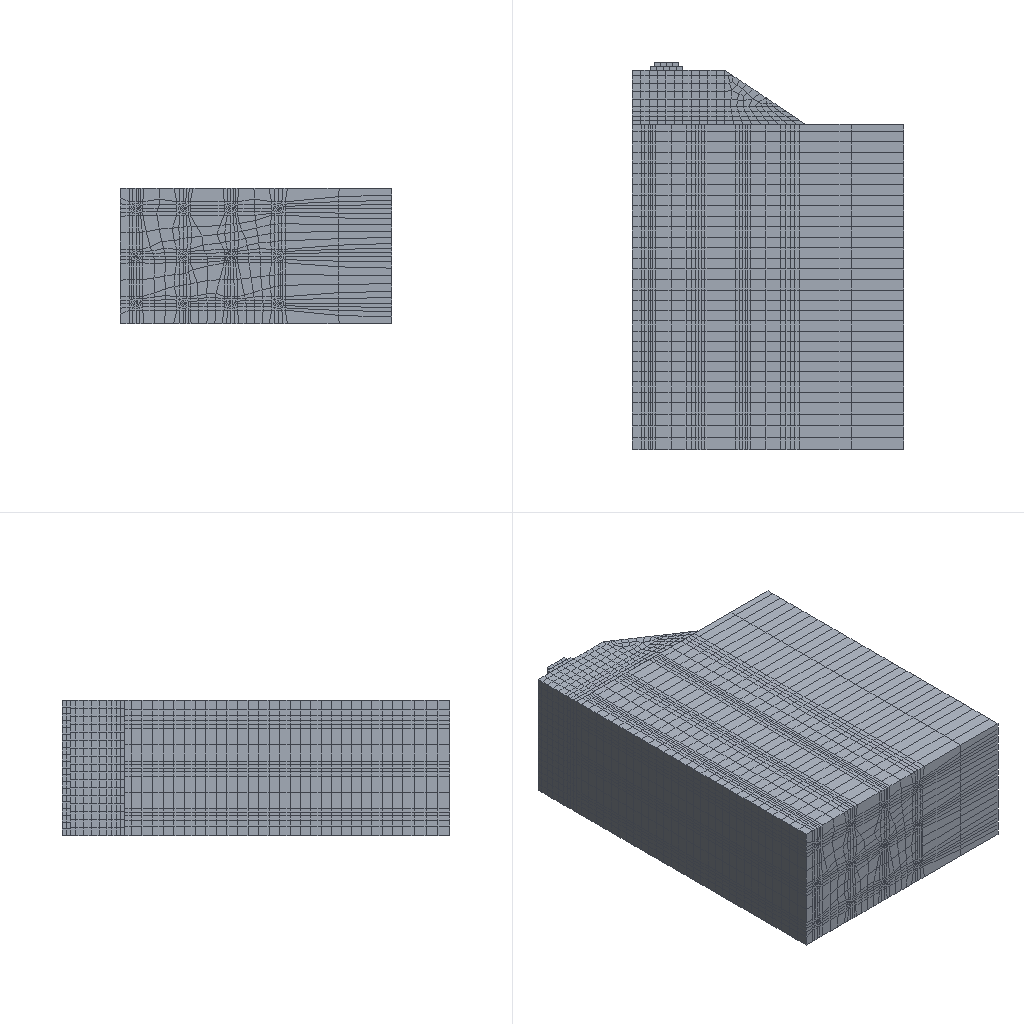Simulation study | abaqus
Set-up summary:
category,name,step,type,value,unit,region
solver,abaqus
solver,version,,,Abaqus/Standard 2020
units,not stated in the deck,,not stated
analysis,deck,,geostatic,geostatic
load_step,Step-geo,Step-geo,geostatic
load_step,Step-ludi,Step-ludi,static
load_step,Step-load,Step-load,static
load_step,requested,,,3
mesh,nodes,,,32812
mesh,elements,,,26703
element_type,C3D8R,,solid,26623
element_type,M3D4R,,membrane,80
load,load commands in deck,,count,2
bc,support commands in deck,,count,3
material,DIZUOBAN,,in results
material,FENSHA,,in results
material,GESHAN,,in results
material,GUIDAOBAN,,in results
material,JICHAUNBIAOCENG,,in results
material,JICHUANDICENG,,in results
material,LUDI,,in results
material,RUANTU1,,in results
material,RUANTU2,,in results
material,RUANTU3,,in results
material,SUISHI,,in results
material,ZHUANG,,in results
check,setup vs results,,match,"per instance, exact: element labels, types and connectivity; labels of the nodes the elements use; coordinates of those nodes at SINGLE_PRECISION in 6 of 6 instance(s)"
Abaqus input file, long lists of numbers shortened:
*Heading
** Job name: Job-1 Model name: Model-1
** Generated by: Abaqus/CAE 2020
*Preprint, echo=NO, model=NO, history=NO, contact=NO
**
** PARTS
**
*Part, name=dizuoban
*Node
      1,   3.7,   4.3,          10.
      2,   3.7,           4.,          10.
** (250 more lines like these left out)
*Element, type=C3D8R
  1,  43,  44,  46,  45,   1,   2,   4,   3
  2,  45,  46,  48,  47,   3,   4,   6,   5
** (98 more lines like these left out)
*Nset, nset=Set-1, generate
   1,  252,    1
*Elset, elset=Set-1, generate
   1,  100,    1
** Section: dizuoban
*Solid Section, elset=Set-1, material=dizuoban
,
*End Part
**
*Part, name=geshan
*Node
      1,           0.,  0.3,           0.
      2,   1.235,  0.3,           0.
** (97 more lines like these left out)
*Element, type=M3D4R
 1,  1,  2, 13, 12
 2,  2,  3, 14, 13
** (78 more lines like these left out)
*Nset, nset=Set-2, generate
  1,  99,   1
*Elset, elset=Set-2, generate
  1,  80,   1
** Section: geshan
*Membrane Section, elset=Set-2, material=geshan
0.003,
*End Part
**
*Part, name=guidaoban
*Node
      1,    3.4,    4.6,          10.
      2,    3.4,   4.3,          10.
** (208 more lines like these left out)
*Element, type=C3D8R
 1,  43,  44,  46,  45,   1,   2,   4,   3
 2,  45,  46,  48,  47,   3,   4,   6,   5
** (78 more lines like these left out)
*Nset, nset=Set-1, generate
   1,  210,    1
*Elset, elset=Set-1, generate
  1,  80,   1
** Section: guidaoban
*Solid Section, elset=Set-1, material=guidaoban
,
*End Part
**
*Part, name=ludi
*Node
      1,   6.8, -0.4,           0.
      2,   6.8, -0.4,          10.
** (3400 more lines like these left out)
*Element, type=C3D8R
  1,    1,   29,  439,   80,   81,  789, 2091,  768
  2,   29,   30,  440,  439,  789,  790, 2092, 2091
** (2752 more lines like these left out)
*Nset, nset=Set-4
    1,    2,    3,    4,   17,   18,   19,   20,   26,   27,   29,   30,   31,   32,   33,   34
   35,   36,   37,   38,   39,   40,   41,   42,   43,   44,   45,   46,   47,   48,   49,   50
** (28 more lines like these left out)
*Elset, elset=Set-4
 1497, 1498, 1499, 1500, 1501, 1502, 1503, 1504, 1505, 1506, 1507, 1508, 1509, 1510, 1511, 1512
 1513, 1514, 1515, 1516, 1517, 1518, 1519, 1520, 1521, 1522, 1523, 1524, 1525, 1526, 1527, 1528
** (11 more lines like these left out)
*Nset, nset=Set-5
    1,    2,    3,    4,    5,    6,    7,    8,   25,   26,   27,   28,   29,   30,   31,   32
   33,   34,   35,   36,   37,   38,   39,   40,   41,   42,   43,   44,   45,   46,   47,   48
** (103 more lines like these left out)
*Elset, elset=Set-5
    1,    2,    3,    4,    5,    6,    7,    8,    9,   10,   11,   12,   13,   14,   15,   16
   17,   18,   19,   20,   21,   22,   23,   24,   25,   26,   27,   28,   29,   30,   31,   32
** (73 more lines like these left out)
*Nset, nset=Set-6
    5,    6,    7,    8,    9,   10,   11,   12,   21,   24,   25,   28,   93,   94,   95,   96
   97,   98,   99,  100,  101,  102,  103,  104,  105,  106,  107,  108,  109,  110,  111,  112
** (69 more lines like these left out)
*Elset, elset=Set-6
  749,  750,  751,  752,  753,  754,  755,  756,  757,  758,  759,  760,  761,  762,  763,  764
  765,  766,  767,  768,  769,  770,  771,  772,  773,  774,  775,  776,  777,  778,  779,  780
** (41 more lines like these left out)
*Nset, nset=Set-7
    9,   10,   11,   12,   13,   14,   15,   16,   21,   22,   23,   24,  149,  150,  151,  152
  153,  154,  155,  156,  157,  158,  159,  160,  161,  162,  163,  164,  165,  166,  167,  168
** (69 more lines like these left out)
*Elset, elset=Set-7
 1123, 1124, 1125, 1126, 1127, 1128, 1129, 1130, 1131, 1132, 1133, 1134, 1135, 1136, 1137, 1138
 1139, 1140, 1141, 1142, 1143, 1144, 1145, 1146, 1147, 1148, 1149, 1150, 1151, 1152, 1153, 1154
** (41 more lines like these left out)
** Section: jichuandiceng
*Solid Section, elset=Set-5, material=jichuandiceng
,
** Section: ludi
*Solid Section, elset=Set-6, material=ludi
,
** Section: suishi
*Solid Section, elset=Set-7, material=suishi
,
** Section: jichuanbiaoceng
*Solid Section, elset=Set-4, material=jichaunbiaoceng
,
*End Part
**
*Part, name=pile
*Node
      1,   8.15,           0.,           8.
      2,   8.15,           0.,         8.25
** (3514 more lines like these left out)
*Element, type=C3D8R
 1, 1647,  375, 1646, 2989,  373,    1,  374, 1645
 2, 1648,  377, 1647, 2989,  376,    2,  373, 1645
** (2206 more lines like these left out)
*Nset, nset=Set-1, generate
    1,  3516,     1
*Elset, elset=Set-1, generate
    1,  2208,     1
** Section: zhuang
*Solid Section, elset=Set-1, material=zhuang
,
*End Part
**
*Part, name=soil-merge
*Node
      1,   12.15,         -19.,          5.5
      2,   12.15,         -19.,           8.
** (25331 more lines like these left out)
*Element, type=C3D8R
  1,  1162,  7498,  7495,     1,  7544, 18528, 18525,  1218
  2,  7498,  7499,  7496,  7495, 18528, 18529, 18526, 18525
** (21479 more lines like these left out)
*Nset, nset=Set-1
     1,     2,     3,     4,     5,     8,     9,    10,    11,    12,    15,    16,    17,    18,    19,    20
    21,    22,    23,    24,    25,    26,    27,    28,    29,    30,    31,    32,    33,    34,    35,    36
** (974 more lines like these left out)
*Elset, elset=Set-1
   443,   444,   445,   446,   447,   448,   449,   450,   451,   452,   453,   454,   455,   456,   457,   458
   459,   460,   461,   462,   463,   464,   465,   466,   467,   468,   469,   470,   471,   472,   473,   474
** (672 more lines like these left out)
*Nset, nset=Set-2
     9,    10,    11,    12,    13,    14,    15,    16,    17,    18,    19,    20,    21,    22,    23,    24
    47,    48,    49,    50,    51,    52,    53,    54,    55,    56,    57,    58,   144,   145,   152,   153
** (328 more lines like these left out)
*Elset, elset=Set-2
   209,   210,   211,   212,   213,   214,   215,   216,   217,   218,   219,   220,   221,   222,   223,   224
   225,   226,   227,   228,   229,   230,   231,   232,   233,   234,   235,   236,   237,   238,   239,   240
** (212 more lines like these left out)
*Nset, nset=Set-3
     1,     2,     3,     4,     5,     6,     7,     8,     9,    10,    11,    12,    13,    14,    15,    16
    41,    42,    43,    44,    45,    46,    47,    48,    49,    50,    51,    52,   143,   144,   151,   152
** (295 more lines like these left out)
*Elset, elset=Set-3
     1,     2,     3,     4,     5,     6,     7,     8,     9,    10,    11,    12,    13,    14,    15,    16
    17,    18,    19,    20,    21,    22,    23,    24,    25,    26,    27,    28,    29,    30,    31,    32
** (188 more lines like these left out)
*Nset, nset=Set-4
     1,     2,     3,     4,     5,     6,     7,     8,    41,    42,    43,    44,    45,    46,    71,    72
    73,    74,    75,    76,    77,    78,    79,    80,    81,    82,    83,    84,    85,    86,    87,    88
** (354 more lines like these left out)
*Elset, elset=Set-4
  1226,  1227,  1228,  1229,  1230,  1231,  1232,  1233,  1234,  1235,  1236,  1237,  1238,  1239,  1240,  1241
  1242,  1243,  1244,  1245,  1246,  1247,  1248,  1249,  1250,  1251,  1252,  1253,  1254,  1255,  1256,  1257
** (265 more lines like these left out)
** Section: ruantu3
*Solid Section, elset=Set-3, material=ruantu3
,
** Section: ruantu2
*Solid Section, elset=Set-2, material=ruantu2
,
** Section: ruantu1
*Solid Section, elset=Set-1, material=ruantu1
,
** Section: fensha
*Solid Section, elset=Set-4, material=fensha
,
*End Part
**
**
** ASSEMBLY
**
*Assembly, name=Assembly
**
*Instance, name=dizuoban-1, part=dizuoban
*End Instance
**
*Instance, name=geshan-1, part=geshan
*End Instance
**
*Instance, name=guidaoban-1, part=guidaoban
*End Instance
**
*Instance, name=ludi-1, part=ludi
          0.,           4.,           0.
*End Instance
**
*Instance, name=pile-1, part=pile
*End Instance
**
*Instance, name=soil-merge-1, part=soil-merge
*End Instance
**
*Nset, nset=Set-1, instance=dizuoban-1, generate
   1,  252,    1
*Nset, nset=Set-1, instance=geshan-1, generate
  1,  99,   1
*Nset, nset=Set-1, instance=ludi-1, generate
    1,  3402,     1
*Nset, nset=Set-1, instance=guidaoban-1, generate
   1,  210,    1
*Nset, nset=Set-1, instance=pile-1, generate
    1,  3516,     1
*Elset, elset=Set-1, instance=dizuoban-1, generate
   1,  100,    1
*Elset, elset=Set-1, instance=geshan-1, generate
  1,  80,   1
*Elset, elset=Set-1, instance=ludi-1, generate
    1,  2754,     1
*Elset, elset=Set-1, instance=guidaoban-1, generate
  1,  80,   1
*Elset, elset=Set-1, instance=pile-1, generate
    1,  2208,     1
*Nset, nset=Set-4, instance=dizuoban-1
   1,   2,  41,  42,  43,  44,  83,  84,  85,  86, 125, 126, 127, 128, 167, 168
 169, 170, 209, 210, 211, 212, 251, 252
*Nset, nset=Set-4, instance=guidaoban-1
   1,   2,  41,  42,  43,  44,  83,  84,  85,  86, 125, 126, 127, 128, 167, 168
 169, 170, 209, 210
*Nset, nset=Set-4, instance=ludi-1
    1,    2,    3,    4,    5,    6,    7,    8,    9,   10,   11,   12,   13,   14,   15,   16
   17,   18,   19,   20,   21,   22,   23,   24,   25,   26,   27,   28,   45,   46,   47,   48
** (22 more lines like these left out)
*Nset, nset=Set-4, instance=soil-merge-1
   155,   156,   157,   158,   159,   160,   161,   162,   163,   166,   167,   168,   170,   171,   190,   192
   193,   196,   197,   200,   201,   204,   206,   207,   209,   212,   213,   216,   375,   378,   381,   384
** (118 more lines like these left out)
*Elset, elset=Set-4, instance=dizuoban-1
   1,  20,  21,  40,  41,  60,  61,  80,  81, 100
*Elset, elset=Set-4, instance=guidaoban-1
  1, 20, 21, 40, 41, 60, 61, 80
*Elset, elset=Set-4, instance=ludi-1
    1,   17,   18,   34,   35,   51,   52,   68,   69,   85,   86,  102,  103,  119,  120,  136
  137,  153,  154,  170,  171,  187,  188,  204,  205,  221,  222,  238,  239,  255,  256,  272
** (19 more lines like these left out)
*Elset, elset=Set-4, instance=soil-merge-1
  2378,  2379,  2386,  2387,  2388,  2389,  2396,  2397,  2398,  2399,  2406,  2407,  2408,  2409,  2416,  2417
  2418,  2419,  2426,  2427,  2428,  2429,  2436,  2437,  2438,  2439,  2446,  2447,  2448,  2449,  2456,  2457
** (111 more lines like these left out)
*Nset, nset=Set-5, instance=ludi-1
    3,    4,    7,    8,   11,   12,   15,   16,   17,   20,   55,   56,   57,   58,   59,   60
   61,   62,   63,   64,   65,   66,   67,   68,   69,   70,   84,   85,   86,   90,   91,   92
** (10 more lines like these left out)
*Nset, nset=Set-5, instance=soil-merge-1
     6,     7,    13,    14,    21,    22,    29,    30,    37,    38,    46,    51,    57,    63,    68,    75
    76,    83,    84,    90,    96,   155,   158,   160,   162,   166,   168,   171,   192,   196,   200,   204
** (86 more lines like these left out)
*Elset, elset=Set-5, instance=ludi-1
  171,  172,  173,  174,  175,  176,  177,  178,  179,  180,  181,  182,  183,  184,  185,  186
  187,  358,  359,  360,  361,  362,  363,  364,  365,  366,  367,  368,  369,  370,  371,  372
** (8 more lines like these left out)
*Elset, elset=Set-5, instance=soil-merge-1
    10,    12,    14,    16,    18,    20,    22,    24,    26,    36,    38,    40,    42,    44,    46,    48
    50,    52,    62,    64,    66,    68,    70,    72,    74,    76,    78,    88,    90,    92,    94,    96
** (80 more lines like these left out)
*Nset, nset=Set-6, instance=soil-merge-1
    79,    80,    81,    82,    83,    84,    85,    86,    93,    94,    95,    96,    97,    98,   169,   170
   171,   172,   173,   174,   176,   177,   178,   179,   180,   182,   183,   184,   185,   186,   188,   213
** (56 more lines like these left out)
*Elset, elset=Set-6, instance=soil-merge-1
  1341,  1342,  1343,  1344,  1345,  1346,  1347,  1348,  1349,  1350,  1351,  1352,  1353,  1354,  1355,  1356
  1357,  1358,  1359,  1360,  1361,  1362,  1363,  1494,  1495,  1496,  1497,  1498,  1499,  1500,  1501,  1502
** (53 more lines like these left out)
*Nset, nset=Set-7, instance=soil-merge-1
     1,     2,     3,     4,     5,     8,     9,    10,    11,    12,    15,    16,    17,    18,    19,    20
    23,    24,    25,    26,    27,    28,    31,    32,    33,    34,    35,    36,    39,    40,    41,    42
** (810 more lines like these left out)
*Elset, elset=Set-7, instance=soil-merge-1
     1,     4,     5,     8,     9,    11,    13,    23,    25,    27,    30,    31,    34,    35,    37,    39
    49,    51,    53,    56,    57,    60,    61,    63,    65,    75,    77,    79,    82,    83,    86,    87
** (888 more lines like these left out)
*Nset, nset=Set-8, instance=soil-merge-1
     1,     2,     3,     4,     5,     8,     9,    10,    11,    12,    15,    16,    17,    18,    19,    20
    23,    24,    25,    26,    27,    28,    31,    32,    33,    34,    35,    36,    39,    40,    41,    42
** (810 more lines like these left out)
*Elset, elset=Set-8, instance=soil-merge-1
     1,     4,     5,     8,     9,    11,    13,    23,    25,    27,    30,    31,    34,    35,    37,    39
    49,    51,    53,    56,    57,    60,    61,    63,    65,    75,    77,    79,    82,    83,    86,    87
** (888 more lines like these left out)
*Nset, nset=Set-9, instance=dizuoban-1, generate
   1,  252,    1
*Nset, nset=Set-9, instance=geshan-1, generate
  1,  99,   1
*Nset, nset=Set-9, instance=ludi-1, generate
    1,  3402,     1
*Nset, nset=Set-9, instance=guidaoban-1, generate
   1,  210,    1
*Elset, elset=Set-9, instance=dizuoban-1, generate
   1,  100,    1
*Elset, elset=Set-9, instance=geshan-1, generate
  1,  80,   1
*Elset, elset=Set-9, instance=ludi-1, generate
    1,  2754,     1
*Elset, elset=Set-9, instance=guidaoban-1, generate
  1,  80,   1
*Nset, nset=Set-10, instance=dizuoban-1, generate
   1,  252,    1
*Nset, nset=Set-10, instance=geshan-1, generate
  1,  99,   1
*Nset, nset=Set-10, instance=ludi-1, generate
    1,  3402,     1
*Nset, nset=Set-10, instance=guidaoban-1, generate
   1,  210,    1
*Elset, elset=Set-10, instance=dizuoban-1, generate
   1,  100,    1
*Elset, elset=Set-10, instance=geshan-1, generate
  1,  80,   1
*Elset, elset=Set-10, instance=ludi-1, generate
    1,  2754,     1
*Elset, elset=Set-10, instance=guidaoban-1, generate
  1,  80,   1
*Nset, nset=m_Set-2, instance=geshan-1, generate
  1,  99,   1
*Elset, elset=m_Set-2, instance=geshan-1, generate
  1,  80,   1
*Nset, nset=s_Set-2, instance=ludi-1, generate
    1,  3402,     1
*Elset, elset=s_Set-2, instance=ludi-1, generate
    1,  2754,     1
*Elset, elset=_Surf-1_S6, internal, instance=guidaoban-1, generate
  1,  80,   1
*Surface, type=ELEMENT, name=Surf-1
_Surf-1_S6, S6
*Elset, elset=_m_Surf-2_S6, internal, instance=dizuoban-1, generate
   1,  100,    1
*Surface, type=ELEMENT, name=m_Surf-2
_m_Surf-2_S6, S6
*Elset, elset=_m_Surf-4_S2, internal, instance=ludi-1, generate
 1497,  1683,     1
*Surface, type=ELEMENT, name=m_Surf-4
_m_Surf-4_S2, S2
*Elset, elset=_m_Surf-6_S3, internal, instance=pile-1
    1,   42,   46,   49,   63,   67,  105,  117,  187,  193,  194,  256,  260,  263,  274,  278
  279,  280,  343,  355,  379,  383,  421,  425,  444,  448,  451,  483,  557,  561,  632,  636
** (6 more lines like these left out)
*Elset, elset=_m_Surf-6_S4, internal, instance=pile-1
    2,   43,   66,  104,  107,  116,  118,  186,  189,  257,  273,  342,  345,  354,  356,  378
  380,  382,  385,  424,  445,  484,  556,  558,  560,  563,  631,  647,  716,  719,  738,  779
** (4 more lines like these left out)
*Elset, elset=_m_Surf-6_S2, internal, instance=pile-1
    5,    6,    7,   50,   51,   52,   53,   57,   58,   59,   69,   70,  109,  110,  119,  120
  121,  264,  265,  266,  267,  347,  348,  357,  358,  359,  363,  364,  365,  369,  370,  371
** (10 more lines like these left out)
*Surface, type=ELEMENT, name=m_Surf-6
_m_Surf-6_S3, S3
_m_Surf-6_S4, S4
_m_Surf-6_S2, S2
*Elset, elset=_m_Surf-8_S2, internal, instance=soil-merge-1
   625,   626,   627,   628,   629,   630,   631,   632,   633,   634,   635,   636,   637,   638,   639,   640
   641,   642,   643,   644,   645,   646,   647,   648,   649,   650,  1203,  1204,  1205,  1206,  1207,  1208
** (22 more lines like these left out)
*Surface, type=ELEMENT, name=m_Surf-8
_m_Surf-8_S2, S2
*Elset, elset=_m_Surf-10_S2, internal, instance=ludi-1, generate
 1310,  1496,     1
*Elset, elset=_m_Surf-10_S6, internal, instance=ludi-1, generate
 1684,  1988,     2
*Surface, type=ELEMENT, name=m_Surf-10
_m_Surf-10_S2, S2
_m_Surf-10_S6, S6
*Elset, elset=_m_Surf-12_S2, internal, instance=soil-merge-1
  1645,  1646,  1647,  1648,  1649,  1825,  1826,  1827,  1828,  1829,  1830,  1831,  2007,  2008,  2009,  2010
  2011,  2012,  2013,  2189,  2190,  2191,  2192,  2193,  2194,  2195,  2371,  2372,  2373,  2374,  2375,  2376
** (17 more lines like these left out)
*Elset, elset=_m_Surf-12_S4, internal, instance=soil-merge-1
   628,   632,  1205,  1208,  1211,  1524,  1529,  1534,  1539,  1544,  1549,  1554,  1559,  1564,  1569,  1574
  1579,  1584,  1589,  1594,  1599,  1604,  1609,  1614,  1619,  1624,  1629,  1634,  1639,  1644,  1649,  1651
** (42 more lines like these left out)
*Elset, elset=_m_Surf-12_S5, internal, instance=soil-merge-1
  1520,  1525,  1530,  1535,  1540,  1545,  1550,  1555,  1560,  1565,  1570,  1575,  1580,  1585,  1590,  1595
  1600,  1605,  1610,  1615,  1620,  1625,  1630,  1635,  1640,  1645,  1832,  1833,  1839,  1840,  1846,  1847
** (85 more lines like these left out)
*Elset, elset=_m_Surf-12_S6, internal, instance=soil-merge-1
   625,   629,   633,   635,   637,   647,   649,  1203,  1206,  1209,  1212,  1214,  1222,  1224,  1652,  1653
  1659,  1660,  1666,  1667,  1673,  1674,  1680,  1681,  1687,  1688,  1694,  1695,  1701,  1702,  1708,  1709
** (55 more lines like these left out)
*Elset, elset=_m_Surf-12_S1, internal, instance=soil-merge-1
  2716,  2717,  2718,  2719,  2720,  2736,  2737,  2738,  2739,  2740,  2812,  2813,  2814,  2815,  2816,  2832
  2833,  2834,  2835,  2836,  2900,  2901,  2902,  2903,  2904,  3258,  3259,  3260,  3261,  3262,  7065,  7066
** (11 more lines like these left out)
*Elset, elset=_m_Surf-12_S3, internal, instance=soil-merge-1
  3280,  3281,  3287,  3288,  3294,  3295,  3301,  3302,  3308,  3309,  3315,  3316,  3322,  3323,  3329,  3330
  3336,  3337,  3343,  3344,  3350,  3351,  3357,  3358,  3364,  3365,  3371,  3372,  3378,  3379,  3385,  3386
** (20 more lines like these left out)
*Surface, type=ELEMENT, name=m_Surf-12
_m_Surf-12_S2, S2
_m_Surf-12_S4, S4
_m_Surf-12_S6, S6
_m_Surf-12_S5, S5
_m_Surf-12_S1, S1
_m_Surf-12_S3, S3
*Elset, elset=_s_Surf-2_S4, internal, instance=guidaoban-1, generate
  1,  80,   1
*Surface, type=ELEMENT, name=s_Surf-2
_s_Surf-2_S4, S4
*Elset, elset=_s_Surf-4_S4, internal, instance=dizuoban-1, generate
   1,  100,    1
*Surface, type=ELEMENT, name=s_Surf-4
_s_Surf-4_S4, S4
*Elset, elset=_s_Surf-6_S2, internal, instance=ludi-1, generate
 1310,  1496,     1
*Elset, elset=_s_Surf-6_S6, internal, instance=ludi-1, generate
 1684,  1988,     2
*Surface, type=ELEMENT, name=s_Surf-6
_s_Surf-6_S2, S2
_s_Surf-6_S6, S6
*Elset, elset=_s_Surf-8_S2, internal, instance=ludi-1, generate
 1310,  1496,     1
*Elset, elset=_s_Surf-8_S6, internal, instance=ludi-1, generate
 1684,  1988,     2
*Surface, type=ELEMENT, name=s_Surf-8
_s_Surf-8_S2, S2
_s_Surf-8_S6, S6
*Elset, elset=_s_Surf-10_S2, internal, instance=soil-merge-1
   625,   626,   627,   628,   629,   630,   631,   632,   633,   634,   635,   636,   637,   638,   639,   640
   641,   642,   643,   644,   645,   646,   647,   648,   649,   650,  1203,  1204,  1205,  1206,  1207,  1208
** (22 more lines like these left out)
*Surface, type=ELEMENT, name=s_Surf-10
_s_Surf-10_S2, S2
*Elset, elset=_s_Surf-12_S4, internal, instance=pile-1
    1,    4,    6,    7,    9,   10,   16,   17,   18,   19,   20,   26,   27,   28,   29,   30
   36,   37,   38,   39,   40,   41,   44,   45,   47,   48,   49,   50,   64,   65,   68,   78
** (50 more lines like these left out)
*Elset, elset=_s_Surf-12_S3, internal, instance=pile-1
    3,    4,    7,    8,    9,   10,   21,   22,   23,   24,   25,   43,   44,   48,   50,   65
   66,   69,   71,   72,   83,   84,   85,   86,   87,   93,   98,   99,  100,  101,  102,  103
** (43 more lines like these left out)
*Elset, elset=_s_Surf-12_S2, internal, instance=pile-1
   10,   11,   16,   21,   47,   48,   63,   64,   65,   66,   71,  112,  185,  186,  187,  188
  191,  192,  193,  195,  200,  205,  261,  262,  275,  276,  277,  280,  350,  390,  421,  422
** (11 more lines like these left out)
*Surface, type=ELEMENT, name=s_Surf-12
_s_Surf-12_S4, S4
_s_Surf-12_S3, S3
_s_Surf-12_S2, S2
** Constraint: Constraint-1
*Embedded Element, host elset=s_Set-2
m_Set-2
*End Assembly
*Amplitude, name=Amp-1
             0.,              0.,              1.,              1.
**
** MATERIALS
**
*Material, name=dizuoban
*Density
2500.,
*Elastic
 2.6e+10, 0.2
*Material, name=fensha
*Density
1800.,
*Elastic
 5e+07, 0.25
*Mohr Coulomb
25., 0.1
*Mohr Coulomb Hardening
25000.,0.
*Material, name=geshan
*Density
1500.,
*Elastic
 8e+08, 0.2
*Material, name=guidaoban
*Density
2500.,
*Elastic
 2.65e+10, 0.2
*Material, name=jichaunbiaoceng
*Density
2200.,
*Elastic
 7e+07, 0.35
*Material, name=jichuandiceng
*Density
2100.,
*Elastic
 5e+07, 0.33
*Material, name=ludi
*Density
1850.,
*Elastic
 9e+07, 0.25
*Material, name=ruantu1
*Density
1640.,
*Elastic
 9.4e+06, 0.35
*Mohr Coulomb
 9.1, 0.1
*Mohr Coulomb Hardening
38000.,0.
*Material, name=ruantu2
*Density
1680.,
*Elastic
 8.6e+06, 0.35
*Mohr Coulomb
 9.1, 0.1
*Mohr Coulomb Hardening
42000.,0.
*Material, name=ruantu3
*Density
1700.,
*Elastic
 9e+06, 0.35
*Mohr Coulomb
 7.7, 0.1
*Mohr Coulomb Hardening
25000.,0.
*Material, name=suishi
*Density
2000.,
*Elastic
 4e+07, 0.2
*Material, name=zhuang
*Density
2350.,
*Elastic
 2e+10, 0.2
**
** INTERACTION PROPERTIES
**
*Surface Interaction, name=IntProp-1
1.,
*Friction, slip tolerance=0.005
 0.3,
*Surface Behavior, pressure-overclosure=HARD
**
** INTERACTIONS
**
** Interaction: Int-jiechu
*Contact Pair, interaction=IntProp-1, type=SURFACE TO SURFACE
m_Surf-2, s_Surf-2
** Interaction: Int-jiechu2
*Contact Pair, interaction=IntProp-1, type=SURFACE TO SURFACE
m_Surf-4, s_Surf-4
** Interaction: Int-jiechu3
*Contact Pair, interaction=IntProp-1, type=SURFACE TO SURFACE, adjust=0.1
m_Surf-6, s_Surf-6
** Interaction: Int-jiechu4
*Contact Pair, interaction=IntProp-1, type=SURFACE TO SURFACE, adjust=0.1
s_Surf-10, m_Surf-10
** Interaction: Int-jiechu5
*Contact Pair, interaction=IntProp-1, type=SURFACE TO SURFACE
s_Surf-12, m_Surf-12
** ----------------------------------------------------------------
**
** STEP: Step-geo
**
*Step, name=Step-geo, nlgeom=YES, inc=1000, unsymm=YES
*Geostatic, utol=0.1
0.01, 1., 1e-05, 1.
**
** BOUNDARY CONDITIONS
**
** Name: [REDACTED] : Displacement/rotation angle
*Boundary
Set-5, 1, 1
** Name: [REDACTED] : Displacement/rotation angle
*Boundary
Set-6, 2, 2
** Name: [REDACTED] : Displacement/rotation angle
*Boundary
Set-4, 3, 3
**
** LOADS
**
** Name: Load-1   Type: Gravity
*Dload
, GRAV, 9.8, 0., -1., 0.
**
** INTERACTIONS
**
** Interaction: Int-del
*Model Change, remove
Set-9,
** Interaction: Int-jiechu
*Model Change, type=CONTACT PAIR, remove
m_Surf-2, s_Surf-2
** Interaction: Int-jiechu2
*Model Change, type=CONTACT PAIR, remove
m_Surf-4, s_Surf-4
** Interaction: Int-jiechu3
*Model Change, type=CONTACT PAIR, remove
m_Surf-6, s_Surf-6
** Interaction: Int-jiechu4
*Model Change, type=CONTACT PAIR, remove
s_Surf-10, m_Surf-10
**
** OUTPUT REQUESTS
**
*Restart, write, frequency=0
**
** FIELD OUTPUT: F-Output-1
**
*Output, field
*Node Output
CF, POR, RF, RM, RT, TF, U, V
*Element Output, directions=YES
CTSHR, E, LE, MISES, MISESMAX, MISESONLY, PE, PEEQ, PEEQMAX, PEEQT, PEMAG, S, SAT, SF, SSAVG, TSHR
VEEQ, VOIDR
*Contact Output
CDISP, CSTRESS
**
** HISTORY OUTPUT: H-Output-1
**
*Output, history, variable=PRESELECT
*End Step
** ----------------------------------------------------------------
**
** STEP: Step-ludi
**
*Step, name=Step-ludi, nlgeom=YES, inc=1000
*Static, stabilize=0.0002, allsdtol=0.05, continue=NO
0.01, 1., 1e-05, 1.
**
** INTERACTIONS
**
** Interaction: Int-add
*Model Change, add
Set-10,
** Interaction: Int-jiechu
*Model Change, type=CONTACT PAIR, add
m_Surf-2, s_Surf-2
** Interaction: Int-jiechu2
*Model Change, type=CONTACT PAIR, add
m_Surf-4, s_Surf-4
** Interaction: Int-jiechu3
*Model Change, type=CONTACT PAIR, add
m_Surf-6, s_Surf-6
** Interaction: Int-jiechu4
*Model Change, type=CONTACT PAIR, add
s_Surf-10, m_Surf-10
**
** OUTPUT REQUESTS
**
*Restart, write, frequency=0
**
** FIELD OUTPUT: F-Output-1
**
*Output, field
*Node Output
CF, RF, RM, RT, TF, U, V
*Element Output, directions=YES
CTSHR, E, LE, MISES, MISESMAX, MISESONLY, PE, PEEQ, PEEQMAX, PEEQT, PEMAG, S, SF, SSAVG, TSHR, VEEQ
*Contact Output
CDISP, CSTRESS
**
** HISTORY OUTPUT: H-Output-1
**
*Output, history, variable=PRESELECT
*End Step
** ----------------------------------------------------------------
**
** STEP: Step-load
**
*Step, name=Step-load, nlgeom=YES, inc=1000
*Static, stabilize=0.0002, allsdtol=0.05, continue=NO
0.01, 1., 1e-05, 1.
**
** LOADS
**
** Name: Load-p   Type: Pressure
*Dsload, amplitude=Amp-1
Surf-1, P, 15000.
**
** OUTPUT REQUESTS
**
*Restart, write, frequency=0
**
** FIELD OUTPUT: F-Output-1
**
*Output, field
*Node Output
CF, RF, RM, RT, TF, U, V
*Element Output, directions=YES
CTSHR, E, LE, MISES, MISESMAX, MISESONLY, PE, PEEQ, PEEQMAX, PEEQT, PEMAG, S, SF, SSAVG, TSHR, VEEQ
*Contact Output
CDISP, CSTRESS
**
** HISTORY OUTPUT: H-Output-1
**
*Output, history, variable=PRESELECT
*End Step
Results summary:
result,step,,completed,increments=27 time=1.0/1.0
result,step,,completed,increments=11 time=1.0/1.0
result,step,,completed,increments=11 time=1.0/1.0
result,analysis,,,static
result,last_loadstep,,,3
result,primary field,,,U
result,reaction total,,FX,-13.903,model units
result,reaction total,,FY,88591838.698,model units
result,reaction total,,FZ,1.656,model units